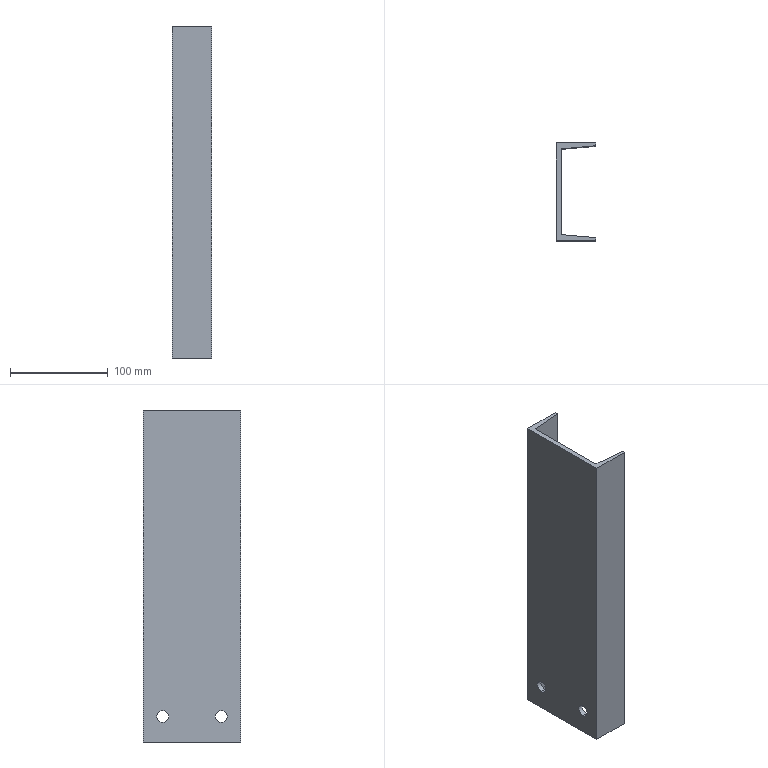Part | STEP file | BCC3 H12_8B | 1 solid | 14 faces | box 40 x 100 x 340 mm | volume 276708 mm3 | plane 10 | cylinder 4 | commonest cylinder face diameters 12 x4
STEP:
#1=CARTESIAN_POINT('',(0.,0.,0.));
#2=DIRECTION('',(0.,0.,1.));
#3=DIRECTION('',(1.,0.,0.));
#4=AXIS2_PLACEMENT_3D('',#1,#2,#3);
#5=CARTESIAN_POINT('',(5.,-30.,-138.));
#6=VERTEX_POINT('',#5);
#7=CARTESIAN_POINT('',(0.,-30.,-138.));
#8=VERTEX_POINT('',#7);
#9=CARTESIAN_POINT('',(10.,-30.,-138.));
#10=DIRECTION('',(-1.,0.,0.));
#11=VECTOR('',#10,1.);
#12=LINE('',#9,#11);
#13=CARTESIAN_POINT('',(10.,-30.,-144.));
#14=DIRECTION('',(-1.,0.,0.));
#15=DIRECTION('',(0.,0.,1.));
#16=AXIS2_PLACEMENT_3D('',#13,#14,#15);
#17=CYLINDRICAL_SURFACE('',#16,6.);
#18=CARTESIAN_POINT('',(6.283,0.));
#19=DIRECTION('',(0.,1.));
#20=VECTOR('',#19,1.);
#21=LINE('',#18,#20);
#22=(GEOMETRIC_REPRESENTATION_CONTEXT(2)PARAMETRIC_REPRESENTATION_CONTEXT()REPRESENTATION_CONTEXT('',''));
#23=DEFINITIONAL_REPRESENTATION('',(#21),#22);
#24=PCURVE('',#17,#23);
#25=CARTESIAN_POINT('',(10.,-30.,-144.));
#26=DIRECTION('',(-1.,0.,0.));
#27=DIRECTION('',(0.,0.,1.));
#28=AXIS2_PLACEMENT_3D('',#25,#26,#27);
#29=CYLINDRICAL_SURFACE('',#28,6.);
#30=CARTESIAN_POINT('',(0.,0.));
#31=DIRECTION('',(0.,1.));
#32=VECTOR('',#31,1.);
#33=LINE('',#30,#32);
#34=(GEOMETRIC_REPRESENTATION_CONTEXT(2)PARAMETRIC_REPRESENTATION_CONTEXT()REPRESENTATION_CONTEXT('',''));
#35=DEFINITIONAL_REPRESENTATION('',(#33),#34);
#36=PCURVE('',#29,#35);
#37=SURFACE_CURVE('',#12,(#24,#36),.PCURVE_S1.);
#38=EDGE_CURVE('',#6,#8,#37,.T.);
#39=ORIENTED_EDGE('',*,*,#38,.T.);
#40=CARTESIAN_POINT('',(0.,-30.,-150.));
#41=VERTEX_POINT('',#40);
#42=CARTESIAN_POINT('',(0.,-30.,-144.));
#43=DIRECTION('',(-1.,0.,0.));
#44=DIRECTION('',(0.,0.,1.));
#45=AXIS2_PLACEMENT_3D('',#42,#43,#44);
#46=CIRCLE('',#45,6.);
#47=CARTESIAN_POINT('',(0.,10.));
#48=DIRECTION('',(1.,0.));
#49=VECTOR('',#48,1.);
#50=LINE('',#47,#49);
#51=(GEOMETRIC_REPRESENTATION_CONTEXT(2)PARAMETRIC_REPRESENTATION_CONTEXT()REPRESENTATION_CONTEXT('',''));
#52=DEFINITIONAL_REPRESENTATION('',(#50),#51);
#53=PCURVE('',#17,#52);
#54=CARTESIAN_POINT('',(0.,50.,170.));
#55=DIRECTION('',(1.,0.,0.));
#56=DIRECTION('',(0.,0.,-1.));
#57=AXIS2_PLACEMENT_3D('',#54,#55,#56);
#58=PLANE('',#57);
#59=CARTESIAN_POINT('',(308.,-80.));
#60=CARTESIAN_POINT('',(308.,-69.608));
#61=CARTESIAN_POINT('',(317.,-74.804));
#62=CARTESIAN_POINT('',(326.,-80.));
#63=CARTESIAN_POINT('',(317.,-85.196));
#64=CARTESIAN_POINT('',(308.,-90.392));
#65=CARTESIAN_POINT('',(308.,-80.));
#66=(BOUNDED_CURVE()B_SPLINE_CURVE(2,(#59,#60,#61,#62,#63,#64,#65),.UNSPECIFIED.,.T.,.F.)B_SPLINE_CURVE_WITH_KNOTS((1,2,2,2,2,1),(-2.094,0.,2.094,4.189,6.283,8.378),.UNSPECIFIED.)CURVE()GEOMETRIC_REPRESENTATION_ITEM()RATIONAL_B_SPLINE_CURVE((1.,0.5,1.,0.5,1.,0.5,1.))REPRESENTATION_ITEM(''));
#67=(GEOMETRIC_REPRESENTATION_CONTEXT(2)PARAMETRIC_REPRESENTATION_CONTEXT()REPRESENTATION_CONTEXT('',''));
#68=DEFINITIONAL_REPRESENTATION('',(#66),#67);
#69=PCURVE('',#58,#68);
#70=SURFACE_CURVE('',#46,(#53,#69),.PCURVE_S1.);
#71=EDGE_CURVE('',#41,#8,#70,.T.);
#72=ORIENTED_EDGE('',*,*,#71,.F.);
#73=CARTESIAN_POINT('',(5.,-30.,-150.));
#74=VERTEX_POINT('',#73);
#75=CARTESIAN_POINT('',(10.,-30.,-150.));
#76=DIRECTION('',(-1.,0.,0.));
#77=VECTOR('',#76,1.);
#78=LINE('',#75,#77);
#79=CARTESIAN_POINT('',(3.142,0.));
#80=DIRECTION('',(0.,1.));
#81=VECTOR('',#80,1.);
#82=LINE('',#79,#81);
#83=(GEOMETRIC_REPRESENTATION_CONTEXT(2)PARAMETRIC_REPRESENTATION_CONTEXT()REPRESENTATION_CONTEXT('',''));
#84=DEFINITIONAL_REPRESENTATION('',(#82),#83);
#85=PCURVE('',#17,#84);
#86=CARTESIAN_POINT('',(3.142,0.));
#87=DIRECTION('',(0.,1.));
#88=VECTOR('',#87,1.);
#89=LINE('',#86,#88);
#90=(GEOMETRIC_REPRESENTATION_CONTEXT(2)PARAMETRIC_REPRESENTATION_CONTEXT()REPRESENTATION_CONTEXT('',''));
#91=DEFINITIONAL_REPRESENTATION('',(#89),#90);
#92=PCURVE('',#29,#91);
#93=SURFACE_CURVE('',#78,(#85,#92),.PCURVE_S1.);
#94=EDGE_CURVE('',#74,#41,#93,.T.);
#95=ORIENTED_EDGE('',*,*,#94,.F.);
#96=CARTESIAN_POINT('',(5.,-30.,-144.));
#97=DIRECTION('',(-1.,0.,0.));
#98=DIRECTION('',(0.,0.,1.));
#99=AXIS2_PLACEMENT_3D('',#96,#97,#98);
#100=CIRCLE('',#99,6.);
#101=CARTESIAN_POINT('',(0.,5.));
#102=DIRECTION('',(1.,0.));
#103=VECTOR('',#102,1.);
#104=LINE('',#101,#103);
#105=(GEOMETRIC_REPRESENTATION_CONTEXT(2)PARAMETRIC_REPRESENTATION_CONTEXT()REPRESENTATION_CONTEXT('',''));
#106=DEFINITIONAL_REPRESENTATION('',(#104),#105);
#107=PCURVE('',#17,#106);
#108=CARTESIAN_POINT('',(5.,-43.938,170.));
#109=DIRECTION('',(-1.,0.,0.));
#110=DIRECTION('',(0.,0.,1.));
#111=AXIS2_PLACEMENT_3D('',#108,#109,#110);
#112=PLANE('',#111);
#113=CARTESIAN_POINT('',(-314.,13.938));
#114=DIRECTION('',(1.,0.));
#115=AXIS2_PLACEMENT_2D('',#113,#114);
#116=CIRCLE('',#115,6.);
#117=(GEOMETRIC_REPRESENTATION_CONTEXT(2)PARAMETRIC_REPRESENTATION_CONTEXT()REPRESENTATION_CONTEXT('',''));
#118=DEFINITIONAL_REPRESENTATION('',(#116),#117);
#119=PCURVE('',#112,#118);
#120=SURFACE_CURVE('',#100,(#107,#119),.PCURVE_S1.);
#121=EDGE_CURVE('',#74,#6,#120,.T.);
#122=ORIENTED_EDGE('',*,*,#121,.T.);
#123=EDGE_LOOP('',(#39,#72,#95,#122));
#124=FACE_BOUND('',#123,.F.);
#125=ADVANCED_FACE('',(#124),#17,.F.);
#126=CARTESIAN_POINT('',(5.,30.,-138.));
#127=VERTEX_POINT('',#126);
#128=CARTESIAN_POINT('',(0.,30.,-138.));
#129=VERTEX_POINT('',#128);
#130=CARTESIAN_POINT('',(10.,30.,-138.));
#131=DIRECTION('',(-1.,0.,0.));
#132=VECTOR('',#131,1.);
#133=LINE('',#130,#132);
#134=CARTESIAN_POINT('',(10.,30.,-144.));
#135=DIRECTION('',(-1.,0.,0.));
#136=DIRECTION('',(0.,0.,1.));
#137=AXIS2_PLACEMENT_3D('',#134,#135,#136);
#138=CYLINDRICAL_SURFACE('',#137,6.);
#139=CARTESIAN_POINT('',(6.283,0.));
#140=DIRECTION('',(0.,1.));
#141=VECTOR('',#140,1.);
#142=LINE('',#139,#141);
#143=(GEOMETRIC_REPRESENTATION_CONTEXT(2)PARAMETRIC_REPRESENTATION_CONTEXT()REPRESENTATION_CONTEXT('',''));
#144=DEFINITIONAL_REPRESENTATION('',(#142),#143);
#145=PCURVE('',#138,#144);
#146=CARTESIAN_POINT('',(10.,30.,-144.));
#147=DIRECTION('',(-1.,0.,0.));
#148=DIRECTION('',(0.,0.,1.));
#149=AXIS2_PLACEMENT_3D('',#146,#147,#148);
#150=CYLINDRICAL_SURFACE('',#149,6.);
#151=CARTESIAN_POINT('',(0.,0.));
#152=DIRECTION('',(0.,1.));
#153=VECTOR('',#152,1.);
#154=LINE('',#151,#153);
#155=(GEOMETRIC_REPRESENTATION_CONTEXT(2)PARAMETRIC_REPRESENTATION_CONTEXT()REPRESENTATION_CONTEXT('',''));
#156=DEFINITIONAL_REPRESENTATION('',(#154),#155);
#157=PCURVE('',#150,#156);
#158=SURFACE_CURVE('',#133,(#145,#157),.PCURVE_S1.);
#159=EDGE_CURVE('',#127,#129,#158,.T.);
#160=ORIENTED_EDGE('',*,*,#159,.T.);
#161=CARTESIAN_POINT('',(0.,30.,-150.));
#162=VERTEX_POINT('',#161);
#163=CARTESIAN_POINT('',(0.,30.,-144.));
#164=DIRECTION('',(-1.,0.,0.));
#165=DIRECTION('',(0.,0.,1.));
#166=AXIS2_PLACEMENT_3D('',#163,#164,#165);
#167=CIRCLE('',#166,6.);
#168=CARTESIAN_POINT('',(0.,10.));
#169=DIRECTION('',(1.,0.));
#170=VECTOR('',#169,1.);
#171=LINE('',#168,#170);
#172=(GEOMETRIC_REPRESENTATION_CONTEXT(2)PARAMETRIC_REPRESENTATION_CONTEXT()REPRESENTATION_CONTEXT('',''));
#173=DEFINITIONAL_REPRESENTATION('',(#171),#172);
#174=PCURVE('',#138,#173);
#175=CARTESIAN_POINT('',(308.,-20.));
#176=CARTESIAN_POINT('',(308.,-9.608));
#177=CARTESIAN_POINT('',(317.,-14.804));
#178=CARTESIAN_POINT('',(326.,-20.));
#179=CARTESIAN_POINT('',(317.,-25.196));
#180=CARTESIAN_POINT('',(308.,-30.392));
#181=CARTESIAN_POINT('',(308.,-20.));
#182=(BOUNDED_CURVE()B_SPLINE_CURVE(2,(#175,#176,#177,#178,#179,#180,#181),.UNSPECIFIED.,.T.,.F.)B_SPLINE_CURVE_WITH_KNOTS((1,2,2,2,2,1),(-2.094,0.,2.094,4.189,6.283,8.378),.UNSPECIFIED.)CURVE()GEOMETRIC_REPRESENTATION_ITEM()RATIONAL_B_SPLINE_CURVE((1.,0.5,1.,0.5,1.,0.5,1.))REPRESENTATION_ITEM(''));
#183=(GEOMETRIC_REPRESENTATION_CONTEXT(2)PARAMETRIC_REPRESENTATION_CONTEXT()REPRESENTATION_CONTEXT('',''));
#184=DEFINITIONAL_REPRESENTATION('',(#182),#183);
#185=PCURVE('',#58,#184);
#186=SURFACE_CURVE('',#167,(#174,#185),.PCURVE_S1.);
#187=EDGE_CURVE('',#162,#129,#186,.T.);
#188=ORIENTED_EDGE('',*,*,#187,.F.);
#189=CARTESIAN_POINT('',(5.,30.,-150.));
#190=VERTEX_POINT('',#189);
#191=CARTESIAN_POINT('',(10.,30.,-150.));
#192=DIRECTION('',(-1.,0.,0.));
#193=VECTOR('',#192,1.);
#194=LINE('',#191,#193);
#195=CARTESIAN_POINT('',(3.142,0.));
#196=DIRECTION('',(0.,1.));
#197=VECTOR('',#196,1.);
#198=LINE('',#195,#197);
#199=(GEOMETRIC_REPRESENTATION_CONTEXT(2)PARAMETRIC_REPRESENTATION_CONTEXT()REPRESENTATION_CONTEXT('',''));
#200=DEFINITIONAL_REPRESENTATION('',(#198),#199);
#201=PCURVE('',#138,#200);
#202=CARTESIAN_POINT('',(3.142,0.));
#203=DIRECTION('',(0.,1.));
#204=VECTOR('',#203,1.);
#205=LINE('',#202,#204);
#206=(GEOMETRIC_REPRESENTATION_CONTEXT(2)PARAMETRIC_REPRESENTATION_CONTEXT()REPRESENTATION_CONTEXT('',''));
#207=DEFINITIONAL_REPRESENTATION('',(#205),#206);
#208=PCURVE('',#150,#207);
#209=SURFACE_CURVE('',#194,(#201,#208),.PCURVE_S1.);
#210=EDGE_CURVE('',#190,#162,#209,.T.);
#211=ORIENTED_EDGE('',*,*,#210,.F.);
#212=CARTESIAN_POINT('',(5.,30.,-144.));
#213=DIRECTION('',(-1.,0.,0.));
#214=DIRECTION('',(0.,0.,1.));
#215=AXIS2_PLACEMENT_3D('',#212,#213,#214);
#216=CIRCLE('',#215,6.);
#217=CARTESIAN_POINT('',(0.,5.));
#218=DIRECTION('',(1.,0.));
#219=VECTOR('',#218,1.);
#220=LINE('',#217,#219);
#221=(GEOMETRIC_REPRESENTATION_CONTEXT(2)PARAMETRIC_REPRESENTATION_CONTEXT()REPRESENTATION_CONTEXT('',''));
#222=DEFINITIONAL_REPRESENTATION('',(#220),#221);
#223=PCURVE('',#138,#222);
#224=CARTESIAN_POINT('',(-314.,73.938));
#225=DIRECTION('',(1.,0.));
#226=AXIS2_PLACEMENT_2D('',#224,#225);
#227=CIRCLE('',#226,6.);
#228=(GEOMETRIC_REPRESENTATION_CONTEXT(2)PARAMETRIC_REPRESENTATION_CONTEXT()REPRESENTATION_CONTEXT('',''));
#229=DEFINITIONAL_REPRESENTATION('',(#227),#228);
#230=PCURVE('',#112,#229);
#231=SURFACE_CURVE('',#216,(#223,#230),.PCURVE_S1.);
#232=EDGE_CURVE('',#190,#127,#231,.T.);
#233=ORIENTED_EDGE('',*,*,#232,.T.);
#234=EDGE_LOOP('',(#160,#188,#211,#233));
#235=FACE_BOUND('',#234,.F.);
#236=ADVANCED_FACE('',(#235),#138,.F.);
#237=CARTESIAN_POINT('',(40.,50.,-170.));
#238=VERTEX_POINT('',#237);
#239=CARTESIAN_POINT('',(0.,50.,-170.));
#240=VERTEX_POINT('',#239);
#241=CARTESIAN_POINT('',(40.,50.,-170.));
#242=DIRECTION('',(-1.,0.,0.));
#243=VECTOR('',#242,1.);
#244=LINE('',#241,#243);
#245=CARTESIAN_POINT('',(40.,50.,170.));
#246=DIRECTION('',(0.,-1.,0.));
#247=DIRECTION('',(1.,0.,0.));
#248=AXIS2_PLACEMENT_3D('',#245,#246,#247);
#249=PLANE('',#248);
#250=CARTESIAN_POINT('',(0.,-340.));
#251=DIRECTION('',(-1.,0.));
#252=VECTOR('',#251,1.);
#253=LINE('',#250,#252);
#254=(GEOMETRIC_REPRESENTATION_CONTEXT(2)PARAMETRIC_REPRESENTATION_CONTEXT()REPRESENTATION_CONTEXT('',''));
#255=DEFINITIONAL_REPRESENTATION('',(#253),#254);
#256=PCURVE('',#249,#255);
#257=CARTESIAN_POINT('',(0.,0.,-170.));
#258=DIRECTION('',(0.,0.,1.));
#259=DIRECTION('',(1.,0.,0.));
#260=AXIS2_PLACEMENT_3D('',#257,#258,#259);
#261=PLANE('',#260);
#262=CARTESIAN_POINT('',(40.,50.));
#263=DIRECTION('',(-1.,0.));
#264=VECTOR('',#263,1.);
#265=LINE('',#262,#264);
#266=(GEOMETRIC_REPRESENTATION_CONTEXT(2)PARAMETRIC_REPRESENTATION_CONTEXT()REPRESENTATION_CONTEXT('',''));
#267=DEFINITIONAL_REPRESENTATION('',(#265),#266);
#268=PCURVE('',#261,#267);
#269=SURFACE_CURVE('',#244,(#256,#268),.PCURVE_S1.);
#270=EDGE_CURVE('',#238,#240,#269,.T.);
#271=ORIENTED_EDGE('',*,*,#270,.T.);
#272=CARTESIAN_POINT('',(0.,50.,170.));
#273=VERTEX_POINT('',#272);
#274=CARTESIAN_POINT('',(0.,50.,170.));
#275=DIRECTION('',(0.,0.,-1.));
#276=VECTOR('',#275,1.);
#277=LINE('',#274,#276);
#278=CARTESIAN_POINT('',(-40.,0.));
#279=DIRECTION('',(0.,-1.));
#280=VECTOR('',#279,1.);
#281=LINE('',#278,#280);
#282=(GEOMETRIC_REPRESENTATION_CONTEXT(2)PARAMETRIC_REPRESENTATION_CONTEXT()REPRESENTATION_CONTEXT('',''));
#283=DEFINITIONAL_REPRESENTATION('',(#281),#282);
#284=PCURVE('',#249,#283);
#285=CARTESIAN_POINT('',(0.,0.));
#286=DIRECTION('',(1.,0.));
#287=VECTOR('',#286,1.);
#288=LINE('',#285,#287);
#289=(GEOMETRIC_REPRESENTATION_CONTEXT(2)PARAMETRIC_REPRESENTATION_CONTEXT()REPRESENTATION_CONTEXT('',''));
#290=DEFINITIONAL_REPRESENTATION('',(#288),#289);
#291=PCURVE('',#58,#290);
#292=SURFACE_CURVE('',#277,(#284,#291),.PCURVE_S1.);
#293=EDGE_CURVE('',#273,#240,#292,.T.);
#294=ORIENTED_EDGE('',*,*,#293,.F.);
#295=CARTESIAN_POINT('',(40.,50.,170.));
#296=VERTEX_POINT('',#295);
#297=CARTESIAN_POINT('',(40.,50.,170.));
#298=DIRECTION('',(-1.,0.,0.));
#299=VECTOR('',#298,1.);
#300=LINE('',#297,#299);
#301=CARTESIAN_POINT('',(0.,0.));
#302=DIRECTION('',(-1.,0.));
#303=VECTOR('',#302,1.);
#304=LINE('',#301,#303);
#305=(GEOMETRIC_REPRESENTATION_CONTEXT(2)PARAMETRIC_REPRESENTATION_CONTEXT()REPRESENTATION_CONTEXT('',''));
#306=DEFINITIONAL_REPRESENTATION('',(#304),#305);
#307=PCURVE('',#249,#306);
#308=CARTESIAN_POINT('',(0.,0.,170.));
#309=DIRECTION('',(0.,0.,1.));
#310=DIRECTION('',(1.,0.,0.));
#311=AXIS2_PLACEMENT_3D('',#308,#309,#310);
#312=PLANE('',#311);
#313=CARTESIAN_POINT('',(40.,50.));
#314=DIRECTION('',(-1.,0.));
#315=VECTOR('',#314,1.);
#316=LINE('',#313,#315);
#317=(GEOMETRIC_REPRESENTATION_CONTEXT(2)PARAMETRIC_REPRESENTATION_CONTEXT()REPRESENTATION_CONTEXT('',''));
#318=DEFINITIONAL_REPRESENTATION('',(#316),#317);
#319=PCURVE('',#312,#318);
#320=SURFACE_CURVE('',#300,(#307,#319),.PCURVE_S1.);
#321=EDGE_CURVE('',#296,#273,#320,.T.);
#322=ORIENTED_EDGE('',*,*,#321,.F.);
#323=CARTESIAN_POINT('',(40.,50.,170.));
#324=DIRECTION('',(0.,0.,-1.));
#325=VECTOR('',#324,1.);
#326=LINE('',#323,#325);
#327=CARTESIAN_POINT('',(0.,0.));
#328=DIRECTION('',(0.,-1.));
#329=VECTOR('',#328,1.);
#330=LINE('',#327,#329);
#331=(GEOMETRIC_REPRESENTATION_CONTEXT(2)PARAMETRIC_REPRESENTATION_CONTEXT()REPRESENTATION_CONTEXT('',''));
#332=DEFINITIONAL_REPRESENTATION('',(#330),#331);
#333=PCURVE('',#249,#332);
#334=CARTESIAN_POINT('',(40.,47.,170.));
#335=DIRECTION('',(-1.,0.,0.));
#336=DIRECTION('',(0.,-1.,0.));
#337=AXIS2_PLACEMENT_3D('',#334,#335,#336);
#338=PLANE('',#337);
#339=CARTESIAN_POINT('',(-3.,0.));
#340=DIRECTION('',(0.,-1.));
#341=VECTOR('',#340,1.);
#342=LINE('',#339,#341);
#343=(GEOMETRIC_REPRESENTATION_CONTEXT(2)PARAMETRIC_REPRESENTATION_CONTEXT()REPRESENTATION_CONTEXT('',''));
#344=DEFINITIONAL_REPRESENTATION('',(#342),#343);
#345=PCURVE('',#338,#344);
#346=SURFACE_CURVE('',#326,(#333,#345),.PCURVE_S1.);
#347=EDGE_CURVE('',#296,#238,#346,.T.);
#348=ORIENTED_EDGE('',*,*,#347,.T.);
#349=EDGE_LOOP('',(#271,#294,#322,#348));
#350=FACE_BOUND('',#349,.T.);
#351=ADVANCED_FACE('',(#350),#249,.F.);
#352=CARTESIAN_POINT('',(0.,-30.,-144.));
#353=DIRECTION('',(-1.,0.,0.));
#354=DIRECTION('',(0.,0.,1.));
#355=AXIS2_PLACEMENT_3D('',#352,#353,#354);
#356=CIRCLE('',#355,6.);
#357=CARTESIAN_POINT('',(308.,-80.));
#358=CARTESIAN_POINT('',(308.,-69.608));
#359=CARTESIAN_POINT('',(317.,-74.804));
#360=CARTESIAN_POINT('',(326.,-80.));
#361=CARTESIAN_POINT('',(317.,-85.196));
#362=CARTESIAN_POINT('',(308.,-90.392));
#363=CARTESIAN_POINT('',(308.,-80.));
#364=(BOUNDED_CURVE()B_SPLINE_CURVE(2,(#357,#358,#359,#360,#361,#362,#363),.UNSPECIFIED.,.T.,.F.)B_SPLINE_CURVE_WITH_KNOTS((1,2,2,2,2,1),(-2.094,0.,2.094,4.189,6.283,8.378),.UNSPECIFIED.)CURVE()GEOMETRIC_REPRESENTATION_ITEM()RATIONAL_B_SPLINE_CURVE((1.,0.5,1.,0.5,1.,0.5,1.))REPRESENTATION_ITEM(''));
#365=(GEOMETRIC_REPRESENTATION_CONTEXT(2)PARAMETRIC_REPRESENTATION_CONTEXT()REPRESENTATION_CONTEXT('',''));
#366=DEFINITIONAL_REPRESENTATION('',(#364),#365);
#367=PCURVE('',#58,#366);
#368=CARTESIAN_POINT('',(0.,10.));
#369=DIRECTION('',(1.,0.));
#370=VECTOR('',#369,1.);
#371=LINE('',#368,#370);
#372=(GEOMETRIC_REPRESENTATION_CONTEXT(2)PARAMETRIC_REPRESENTATION_CONTEXT()REPRESENTATION_CONTEXT('',''));
#373=DEFINITIONAL_REPRESENTATION('',(#371),#372);
#374=PCURVE('',#29,#373);
#375=SURFACE_CURVE('',#356,(#367,#374),.PCURVE_S1.);
#376=EDGE_CURVE('',#8,#41,#375,.T.);
#377=ORIENTED_EDGE('',*,*,#376,.F.);
#378=ORIENTED_EDGE('',*,*,#71,.F.);
#379=EDGE_LOOP('',(#377,#378));
#380=FACE_BOUND('',#379,.T.);
#381=CARTESIAN_POINT('',(0.,30.,-144.));
#382=DIRECTION('',(-1.,0.,0.));
#383=DIRECTION('',(0.,0.,1.));
#384=AXIS2_PLACEMENT_3D('',#381,#382,#383);
#385=CIRCLE('',#384,6.);
#386=CARTESIAN_POINT('',(308.,-20.));
#387=CARTESIAN_POINT('',(308.,-9.608));
#388=CARTESIAN_POINT('',(317.,-14.804));
#389=CARTESIAN_POINT('',(326.,-20.));
#390=CARTESIAN_POINT('',(317.,-25.196));
#391=CARTESIAN_POINT('',(308.,-30.392));
#392=CARTESIAN_POINT('',(308.,-20.));
#393=(BOUNDED_CURVE()B_SPLINE_CURVE(2,(#386,#387,#388,#389,#390,#391,#392),.UNSPECIFIED.,.T.,.F.)B_SPLINE_CURVE_WITH_KNOTS((1,2,2,2,2,1),(-2.094,0.,2.094,4.189,6.283,8.378),.UNSPECIFIED.)CURVE()GEOMETRIC_REPRESENTATION_ITEM()RATIONAL_B_SPLINE_CURVE((1.,0.5,1.,0.5,1.,0.5,1.))REPRESENTATION_ITEM(''));
#394=(GEOMETRIC_REPRESENTATION_CONTEXT(2)PARAMETRIC_REPRESENTATION_CONTEXT()REPRESENTATION_CONTEXT('',''));
#395=DEFINITIONAL_REPRESENTATION('',(#393),#394);
#396=PCURVE('',#58,#395);
#397=CARTESIAN_POINT('',(0.,10.));
#398=DIRECTION('',(1.,0.));
#399=VECTOR('',#398,1.);
#400=LINE('',#397,#399);
#401=(GEOMETRIC_REPRESENTATION_CONTEXT(2)PARAMETRIC_REPRESENTATION_CONTEXT()REPRESENTATION_CONTEXT('',''));
#402=DEFINITIONAL_REPRESENTATION('',(#400),#401);
#403=PCURVE('',#150,#402);
#404=SURFACE_CURVE('',#385,(#396,#403),.PCURVE_S1.);
#405=EDGE_CURVE('',#129,#162,#404,.T.);
#406=ORIENTED_EDGE('',*,*,#405,.F.);
#407=ORIENTED_EDGE('',*,*,#187,.F.);
#408=EDGE_LOOP('',(#406,#407));
#409=FACE_BOUND('',#408,.T.);
#410=CARTESIAN_POINT('',(0.,-50.,-170.));
#411=VERTEX_POINT('',#410);
#412=CARTESIAN_POINT('',(0.,50.,-170.));
#413=DIRECTION('',(0.,-1.,0.));
#414=VECTOR('',#413,1.);
#415=LINE('',#412,#414);
#416=CARTESIAN_POINT('',(340.,0.));
#417=DIRECTION('',(0.,-1.));
#418=VECTOR('',#417,1.);
#419=LINE('',#416,#418);
#420=(GEOMETRIC_REPRESENTATION_CONTEXT(2)PARAMETRIC_REPRESENTATION_CONTEXT()REPRESENTATION_CONTEXT('',''));
#421=DEFINITIONAL_REPRESENTATION('',(#419),#420);
#422=PCURVE('',#58,#421);
#423=CARTESIAN_POINT('',(0.,50.));
#424=DIRECTION('',(0.,-1.));
#425=VECTOR('',#424,1.);
#426=LINE('',#423,#425);
#427=(GEOMETRIC_REPRESENTATION_CONTEXT(2)PARAMETRIC_REPRESENTATION_CONTEXT()REPRESENTATION_CONTEXT('',''));
#428=DEFINITIONAL_REPRESENTATION('',(#426),#427);
#429=PCURVE('',#261,#428);
#430=SURFACE_CURVE('',#415,(#422,#429),.PCURVE_S1.);
#431=EDGE_CURVE('',#240,#411,#430,.T.);
#432=ORIENTED_EDGE('',*,*,#431,.T.);
#433=CARTESIAN_POINT('',(0.,-50.,170.));
#434=VERTEX_POINT('',#433);
#435=CARTESIAN_POINT('',(0.,-50.,170.));
#436=DIRECTION('',(0.,0.,-1.));
#437=VECTOR('',#436,1.);
#438=LINE('',#435,#437);
#439=CARTESIAN_POINT('',(0.,-100.));
#440=DIRECTION('',(1.,0.));
#441=VECTOR('',#440,1.);
#442=LINE('',#439,#441);
#443=(GEOMETRIC_REPRESENTATION_CONTEXT(2)PARAMETRIC_REPRESENTATION_CONTEXT()REPRESENTATION_CONTEXT('',''));
#444=DEFINITIONAL_REPRESENTATION('',(#442),#443);
#445=PCURVE('',#58,#444);
#446=CARTESIAN_POINT('',(0.,-50.,170.));
#447=DIRECTION('',(0.,1.,0.));
#448=DIRECTION('',(-1.,0.,0.));
#449=AXIS2_PLACEMENT_3D('',#446,#447,#448);
#450=PLANE('',#449);
#451=CARTESIAN_POINT('',(0.,0.));
#452=DIRECTION('',(0.,-1.));
#453=VECTOR('',#452,1.);
#454=LINE('',#451,#453);
#455=(GEOMETRIC_REPRESENTATION_CONTEXT(2)PARAMETRIC_REPRESENTATION_CONTEXT()REPRESENTATION_CONTEXT('',''));
#456=DEFINITIONAL_REPRESENTATION('',(#454),#455);
#457=PCURVE('',#450,#456);
#458=SURFACE_CURVE('',#438,(#445,#457),.PCURVE_S1.);
#459=EDGE_CURVE('',#434,#411,#458,.T.);
#460=ORIENTED_EDGE('',*,*,#459,.F.);
#461=CARTESIAN_POINT('',(0.,50.,170.));
#462=DIRECTION('',(0.,-1.,0.));
#463=VECTOR('',#462,1.);
#464=LINE('',#461,#463);
#465=CARTESIAN_POINT('',(0.,0.));
#466=DIRECTION('',(0.,-1.));
#467=VECTOR('',#466,1.);
#468=LINE('',#465,#467);
#469=(GEOMETRIC_REPRESENTATION_CONTEXT(2)PARAMETRIC_REPRESENTATION_CONTEXT()REPRESENTATION_CONTEXT('',''));
#470=DEFINITIONAL_REPRESENTATION('',(#468),#469);
#471=PCURVE('',#58,#470);
#472=CARTESIAN_POINT('',(0.,50.));
#473=DIRECTION('',(0.,-1.));
#474=VECTOR('',#473,1.);
#475=LINE('',#472,#474);
#476=(GEOMETRIC_REPRESENTATION_CONTEXT(2)PARAMETRIC_REPRESENTATION_CONTEXT()REPRESENTATION_CONTEXT('',''));
#477=DEFINITIONAL_REPRESENTATION('',(#475),#476);
#478=PCURVE('',#312,#477);
#479=SURFACE_CURVE('',#464,(#471,#478),.PCURVE_S1.);
#480=EDGE_CURVE('',#273,#434,#479,.T.);
#481=ORIENTED_EDGE('',*,*,#480,.F.);
#482=ORIENTED_EDGE('',*,*,#293,.T.);
#483=EDGE_LOOP('',(#432,#460,#481,#482));
#484=FACE_BOUND('',#483,.T.);
#485=ADVANCED_FACE('',(#380,#409,#484),#58,.F.);
#486=CARTESIAN_POINT('',(40.,-50.,-170.));
#487=VERTEX_POINT('',#486);
#488=CARTESIAN_POINT('',(0.,-50.,-170.));
#489=DIRECTION('',(1.,0.,0.));
#490=VECTOR('',#489,1.);
#491=LINE('',#488,#490);
#492=CARTESIAN_POINT('',(0.,-340.));
#493=DIRECTION('',(-1.,0.));
#494=VECTOR('',#493,1.);
#495=LINE('',#492,#494);
#496=(GEOMETRIC_REPRESENTATION_CONTEXT(2)PARAMETRIC_REPRESENTATION_CONTEXT()REPRESENTATION_CONTEXT('',''));
#497=DEFINITIONAL_REPRESENTATION('',(#495),#496);
#498=PCURVE('',#450,#497);
#499=CARTESIAN_POINT('',(0.,-50.));
#500=DIRECTION('',(1.,0.));
#501=VECTOR('',#500,1.);
#502=LINE('',#499,#501);
#503=(GEOMETRIC_REPRESENTATION_CONTEXT(2)PARAMETRIC_REPRESENTATION_CONTEXT()REPRESENTATION_CONTEXT('',''));
#504=DEFINITIONAL_REPRESENTATION('',(#502),#503);
#505=PCURVE('',#261,#504);
#506=SURFACE_CURVE('',#491,(#498,#505),.PCURVE_S1.);
#507=EDGE_CURVE('',#411,#487,#506,.T.);
#508=ORIENTED_EDGE('',*,*,#507,.T.);
#509=CARTESIAN_POINT('',(40.,-50.,170.));
#510=VERTEX_POINT('',#509);
#511=CARTESIAN_POINT('',(40.,-50.,170.));
#512=DIRECTION('',(0.,0.,-1.));
#513=VECTOR('',#512,1.);
#514=LINE('',#511,#513);
#515=CARTESIAN_POINT('',(-40.,0.));
#516=DIRECTION('',(0.,-1.));
#517=VECTOR('',#516,1.);
#518=LINE('',#515,#517);
#519=(GEOMETRIC_REPRESENTATION_CONTEXT(2)PARAMETRIC_REPRESENTATION_CONTEXT()REPRESENTATION_CONTEXT('',''));
#520=DEFINITIONAL_REPRESENTATION('',(#518),#519);
#521=PCURVE('',#450,#520);
#522=CARTESIAN_POINT('',(40.,-50.,170.));
#523=DIRECTION('',(-1.,0.,0.));
#524=DIRECTION('',(0.,-1.,0.));
#525=AXIS2_PLACEMENT_3D('',#522,#523,#524);
#526=PLANE('',#525);
#527=CARTESIAN_POINT('',(0.,0.));
#528=DIRECTION('',(0.,-1.));
#529=VECTOR('',#528,1.);
#530=LINE('',#527,#529);
#531=(GEOMETRIC_REPRESENTATION_CONTEXT(2)PARAMETRIC_REPRESENTATION_CONTEXT()REPRESENTATION_CONTEXT('',''));
#532=DEFINITIONAL_REPRESENTATION('',(#530),#531);
#533=PCURVE('',#526,#532);
#534=SURFACE_CURVE('',#514,(#521,#533),.PCURVE_S1.);
#535=EDGE_CURVE('',#510,#487,#534,.T.);
#536=ORIENTED_EDGE('',*,*,#535,.F.);
#537=CARTESIAN_POINT('',(0.,-50.,170.));
#538=DIRECTION('',(1.,0.,0.));
#539=VECTOR('',#538,1.);
#540=LINE('',#537,#539);
#541=CARTESIAN_POINT('',(0.,0.));
#542=DIRECTION('',(-1.,0.));
#543=VECTOR('',#542,1.);
#544=LINE('',#541,#543);
#545=(GEOMETRIC_REPRESENTATION_CONTEXT(2)PARAMETRIC_REPRESENTATION_CONTEXT()REPRESENTATION_CONTEXT('',''));
#546=DEFINITIONAL_REPRESENTATION('',(#544),#545);
#547=PCURVE('',#450,#546);
#548=CARTESIAN_POINT('',(0.,-50.));
#549=DIRECTION('',(1.,0.));
#550=VECTOR('',#549,1.);
#551=LINE('',#548,#550);
#552=(GEOMETRIC_REPRESENTATION_CONTEXT(2)PARAMETRIC_REPRESENTATION_CONTEXT()REPRESENTATION_CONTEXT('',''));
#553=DEFINITIONAL_REPRESENTATION('',(#551),#552);
#554=PCURVE('',#312,#553);
#555=SURFACE_CURVE('',#540,(#547,#554),.PCURVE_S1.);
#556=EDGE_CURVE('',#434,#510,#555,.T.);
#557=ORIENTED_EDGE('',*,*,#556,.F.);
#558=ORIENTED_EDGE('',*,*,#459,.T.);
#559=EDGE_LOOP('',(#508,#536,#557,#558));
#560=FACE_BOUND('',#559,.T.);
#561=ADVANCED_FACE('',(#560),#450,.F.);
#562=CARTESIAN_POINT('',(40.,-47.,-170.));
#563=VERTEX_POINT('',#562);
#564=CARTESIAN_POINT('',(40.,-50.,-170.));
#565=DIRECTION('',(0.,1.,0.));
#566=VECTOR('',#565,1.);
#567=LINE('',#564,#566);
#568=CARTESIAN_POINT('',(0.,-340.));
#569=DIRECTION('',(-1.,0.));
#570=VECTOR('',#569,1.);
#571=LINE('',#568,#570);
#572=(GEOMETRIC_REPRESENTATION_CONTEXT(2)PARAMETRIC_REPRESENTATION_CONTEXT()REPRESENTATION_CONTEXT('',''));
#573=DEFINITIONAL_REPRESENTATION('',(#571),#572);
#574=PCURVE('',#526,#573);
#575=CARTESIAN_POINT('',(40.,-50.));
#576=DIRECTION('',(0.,1.));
#577=VECTOR('',#576,1.);
#578=LINE('',#575,#577);
#579=(GEOMETRIC_REPRESENTATION_CONTEXT(2)PARAMETRIC_REPRESENTATION_CONTEXT()REPRESENTATION_CONTEXT('',''));
#580=DEFINITIONAL_REPRESENTATION('',(#578),#579);
#581=PCURVE('',#261,#580);
#582=SURFACE_CURVE('',#567,(#574,#581),.PCURVE_S1.);
#583=EDGE_CURVE('',#487,#563,#582,.T.);
#584=ORIENTED_EDGE('',*,*,#583,.T.);
#585=CARTESIAN_POINT('',(40.,-47.,170.));
#586=VERTEX_POINT('',#585);
#587=CARTESIAN_POINT('',(40.,-47.,170.));
#588=DIRECTION('',(0.,0.,-1.));
#589=VECTOR('',#588,1.);
#590=LINE('',#587,#589);
#591=CARTESIAN_POINT('',(-3.,0.));
#592=DIRECTION('',(0.,-1.));
#593=VECTOR('',#592,1.);
#594=LINE('',#591,#593);
#595=(GEOMETRIC_REPRESENTATION_CONTEXT(2)PARAMETRIC_REPRESENTATION_CONTEXT()REPRESENTATION_CONTEXT('',''));
#596=DEFINITIONAL_REPRESENTATION('',(#594),#595);
#597=PCURVE('',#526,#596);
#598=CARTESIAN_POINT('',(40.,-47.,170.));
#599=DIRECTION('',(-0.08716,-0.9962,0.));
#600=DIRECTION('',(0.9962,-0.08716,0.));
#601=AXIS2_PLACEMENT_3D('',#598,#599,#600);
#602=PLANE('',#601);
#603=CARTESIAN_POINT('',(0.,0.));
#604=DIRECTION('',(0.,-1.));
#605=VECTOR('',#604,1.);
#606=LINE('',#603,#605);
#607=(GEOMETRIC_REPRESENTATION_CONTEXT(2)PARAMETRIC_REPRESENTATION_CONTEXT()REPRESENTATION_CONTEXT('',''));
#608=DEFINITIONAL_REPRESENTATION('',(#606),#607);
#609=PCURVE('',#602,#608);
#610=SURFACE_CURVE('',#590,(#597,#609),.PCURVE_S1.);
#611=EDGE_CURVE('',#586,#563,#610,.T.);
#612=ORIENTED_EDGE('',*,*,#611,.F.);
#613=CARTESIAN_POINT('',(40.,-50.,170.));
#614=DIRECTION('',(0.,1.,0.));
#615=VECTOR('',#614,1.);
#616=LINE('',#613,#615);
#617=CARTESIAN_POINT('',(0.,0.));
#618=DIRECTION('',(-1.,0.));
#619=VECTOR('',#618,1.);
#620=LINE('',#617,#619);
#621=(GEOMETRIC_REPRESENTATION_CONTEXT(2)PARAMETRIC_REPRESENTATION_CONTEXT()REPRESENTATION_CONTEXT('',''));
#622=DEFINITIONAL_REPRESENTATION('',(#620),#621);
#623=PCURVE('',#526,#622);
#624=CARTESIAN_POINT('',(40.,-50.));
#625=DIRECTION('',(0.,1.));
#626=VECTOR('',#625,1.);
#627=LINE('',#624,#626);
#628=(GEOMETRIC_REPRESENTATION_CONTEXT(2)PARAMETRIC_REPRESENTATION_CONTEXT()REPRESENTATION_CONTEXT('',''));
#629=DEFINITIONAL_REPRESENTATION('',(#627),#628);
#630=PCURVE('',#312,#629);
#631=SURFACE_CURVE('',#616,(#623,#630),.PCURVE_S1.);
#632=EDGE_CURVE('',#510,#586,#631,.T.);
#633=ORIENTED_EDGE('',*,*,#632,.F.);
#634=ORIENTED_EDGE('',*,*,#535,.T.);
#635=EDGE_LOOP('',(#584,#612,#633,#634));
#636=FACE_BOUND('',#635,.T.);
#637=ADVANCED_FACE('',(#636),#526,.F.);
#638=CARTESIAN_POINT('',(5.,-43.938,-170.));
#639=VERTEX_POINT('',#638);
#640=CARTESIAN_POINT('',(40.,-47.,-170.));
#641=DIRECTION('',(-0.9962,0.08716,0.));
#642=VECTOR('',#641,1.);
#643=LINE('',#640,#642);
#644=CARTESIAN_POINT('',(0.,-340.));
#645=DIRECTION('',(-1.,0.));
#646=VECTOR('',#645,1.);
#647=LINE('',#644,#646);
#648=(GEOMETRIC_REPRESENTATION_CONTEXT(2)PARAMETRIC_REPRESENTATION_CONTEXT()REPRESENTATION_CONTEXT('',''));
#649=DEFINITIONAL_REPRESENTATION('',(#647),#648);
#650=PCURVE('',#602,#649);
#651=CARTESIAN_POINT('',(40.,-47.));
#652=DIRECTION('',(-0.9962,0.08716));
#653=VECTOR('',#652,1.);
#654=LINE('',#651,#653);
#655=(GEOMETRIC_REPRESENTATION_CONTEXT(2)PARAMETRIC_REPRESENTATION_CONTEXT()REPRESENTATION_CONTEXT('',''));
#656=DEFINITIONAL_REPRESENTATION('',(#654),#655);
#657=PCURVE('',#261,#656);
#658=SURFACE_CURVE('',#643,(#650,#657),.PCURVE_S1.);
#659=EDGE_CURVE('',#563,#639,#658,.T.);
#660=ORIENTED_EDGE('',*,*,#659,.T.);
#661=CARTESIAN_POINT('',(5.,-43.938,170.));
#662=VERTEX_POINT('',#661);
#663=CARTESIAN_POINT('',(5.,-43.938,170.));
#664=DIRECTION('',(0.,0.,-1.));
#665=VECTOR('',#664,1.);
#666=LINE('',#663,#665);
#667=CARTESIAN_POINT('',(-35.134,0.));
#668=DIRECTION('',(0.,-1.));
#669=VECTOR('',#668,1.);
#670=LINE('',#667,#669);
#671=(GEOMETRIC_REPRESENTATION_CONTEXT(2)PARAMETRIC_REPRESENTATION_CONTEXT()REPRESENTATION_CONTEXT('',''));
#672=DEFINITIONAL_REPRESENTATION('',(#670),#671);
#673=PCURVE('',#602,#672);
#674=CARTESIAN_POINT('',(0.,0.));
#675=DIRECTION('',(-1.,0.));
#676=VECTOR('',#675,1.);
#677=LINE('',#674,#676);
#678=(GEOMETRIC_REPRESENTATION_CONTEXT(2)PARAMETRIC_REPRESENTATION_CONTEXT()REPRESENTATION_CONTEXT('',''));
#679=DEFINITIONAL_REPRESENTATION('',(#677),#678);
#680=PCURVE('',#112,#679);
#681=SURFACE_CURVE('',#666,(#673,#680),.PCURVE_S1.);
#682=EDGE_CURVE('',#662,#639,#681,.T.);
#683=ORIENTED_EDGE('',*,*,#682,.F.);
#684=CARTESIAN_POINT('',(40.,-47.,170.));
#685=DIRECTION('',(-0.9962,0.08716,0.));
#686=VECTOR('',#685,1.);
#687=LINE('',#684,#686);
#688=CARTESIAN_POINT('',(0.,0.));
#689=DIRECTION('',(-1.,0.));
#690=VECTOR('',#689,1.);
#691=LINE('',#688,#690);
#692=(GEOMETRIC_REPRESENTATION_CONTEXT(2)PARAMETRIC_REPRESENTATION_CONTEXT()REPRESENTATION_CONTEXT('',''));
#693=DEFINITIONAL_REPRESENTATION('',(#691),#692);
#694=PCURVE('',#602,#693);
#695=CARTESIAN_POINT('',(40.,-47.));
#696=DIRECTION('',(-0.9962,0.08716));
#697=VECTOR('',#696,1.);
#698=LINE('',#695,#697);
#699=(GEOMETRIC_REPRESENTATION_CONTEXT(2)PARAMETRIC_REPRESENTATION_CONTEXT()REPRESENTATION_CONTEXT('',''));
#700=DEFINITIONAL_REPRESENTATION('',(#698),#699);
#701=PCURVE('',#312,#700);
#702=SURFACE_CURVE('',#687,(#694,#701),.PCURVE_S1.);
#703=EDGE_CURVE('',#586,#662,#702,.T.);
#704=ORIENTED_EDGE('',*,*,#703,.F.);
#705=ORIENTED_EDGE('',*,*,#611,.T.);
#706=EDGE_LOOP('',(#660,#683,#704,#705));
#707=FACE_BOUND('',#706,.T.);
#708=ADVANCED_FACE('',(#707),#602,.F.);
#709=CARTESIAN_POINT('',(5.,-30.,-144.));
#710=DIRECTION('',(-1.,0.,0.));
#711=DIRECTION('',(0.,0.,1.));
#712=AXIS2_PLACEMENT_3D('',#709,#710,#711);
#713=CIRCLE('',#712,6.);
#714=CARTESIAN_POINT('',(-314.,13.938));
#715=DIRECTION('',(1.,0.));
#716=AXIS2_PLACEMENT_2D('',#714,#715);
#717=CIRCLE('',#716,6.);
#718=(GEOMETRIC_REPRESENTATION_CONTEXT(2)PARAMETRIC_REPRESENTATION_CONTEXT()REPRESENTATION_CONTEXT('',''));
#719=DEFINITIONAL_REPRESENTATION('',(#717),#718);
#720=PCURVE('',#112,#719);
#721=CARTESIAN_POINT('',(0.,5.));
#722=DIRECTION('',(1.,0.));
#723=VECTOR('',#722,1.);
#724=LINE('',#721,#723);
#725=(GEOMETRIC_REPRESENTATION_CONTEXT(2)PARAMETRIC_REPRESENTATION_CONTEXT()REPRESENTATION_CONTEXT('',''));
#726=DEFINITIONAL_REPRESENTATION('',(#724),#725);
#727=PCURVE('',#29,#726);
#728=SURFACE_CURVE('',#713,(#720,#727),.PCURVE_S1.);
#729=EDGE_CURVE('',#6,#74,#728,.T.);
#730=ORIENTED_EDGE('',*,*,#729,.T.);
#731=ORIENTED_EDGE('',*,*,#121,.T.);
#732=EDGE_LOOP('',(#730,#731));
#733=FACE_BOUND('',#732,.T.);
#734=CARTESIAN_POINT('',(5.,30.,-144.));
#735=DIRECTION('',(-1.,0.,0.));
#736=DIRECTION('',(0.,0.,1.));
#737=AXIS2_PLACEMENT_3D('',#734,#735,#736);
#738=CIRCLE('',#737,6.);
#739=CARTESIAN_POINT('',(-314.,73.938));
#740=DIRECTION('',(1.,0.));
#741=AXIS2_PLACEMENT_2D('',#739,#740);
#742=CIRCLE('',#741,6.);
#743=(GEOMETRIC_REPRESENTATION_CONTEXT(2)PARAMETRIC_REPRESENTATION_CONTEXT()REPRESENTATION_CONTEXT('',''));
#744=DEFINITIONAL_REPRESENTATION('',(#742),#743);
#745=PCURVE('',#112,#744);
#746=CARTESIAN_POINT('',(0.,5.));
#747=DIRECTION('',(1.,0.));
#748=VECTOR('',#747,1.);
#749=LINE('',#746,#748);
#750=(GEOMETRIC_REPRESENTATION_CONTEXT(2)PARAMETRIC_REPRESENTATION_CONTEXT()REPRESENTATION_CONTEXT('',''));
#751=DEFINITIONAL_REPRESENTATION('',(#749),#750);
#752=PCURVE('',#150,#751);
#753=SURFACE_CURVE('',#738,(#745,#752),.PCURVE_S1.);
#754=EDGE_CURVE('',#127,#190,#753,.T.);
#755=ORIENTED_EDGE('',*,*,#754,.T.);
#756=ORIENTED_EDGE('',*,*,#232,.T.);
#757=EDGE_LOOP('',(#755,#756));
#758=FACE_BOUND('',#757,.T.);
#759=CARTESIAN_POINT('',(5.,43.938,-170.));
#760=VERTEX_POINT('',#759);
#761=CARTESIAN_POINT('',(5.,-43.938,-170.));
#762=DIRECTION('',(0.,1.,0.));
#763=VECTOR('',#762,1.);
#764=LINE('',#761,#763);
#765=CARTESIAN_POINT('',(-340.,0.));
#766=DIRECTION('',(0.,1.));
#767=VECTOR('',#766,1.);
#768=LINE('',#765,#767);
#769=(GEOMETRIC_REPRESENTATION_CONTEXT(2)PARAMETRIC_REPRESENTATION_CONTEXT()REPRESENTATION_CONTEXT('',''));
#770=DEFINITIONAL_REPRESENTATION('',(#768),#769);
#771=PCURVE('',#112,#770);
#772=CARTESIAN_POINT('',(5.,-43.938));
#773=DIRECTION('',(0.,1.));
#774=VECTOR('',#773,1.);
#775=LINE('',#772,#774);
#776=(GEOMETRIC_REPRESENTATION_CONTEXT(2)PARAMETRIC_REPRESENTATION_CONTEXT()REPRESENTATION_CONTEXT('',''));
#777=DEFINITIONAL_REPRESENTATION('',(#775),#776);
#778=PCURVE('',#261,#777);
#779=SURFACE_CURVE('',#764,(#771,#778),.PCURVE_S1.);
#780=EDGE_CURVE('',#639,#760,#779,.T.);
#781=ORIENTED_EDGE('',*,*,#780,.T.);
#782=CARTESIAN_POINT('',(5.,43.938,170.));
#783=VERTEX_POINT('',#782);
#784=CARTESIAN_POINT('',(5.,43.938,170.));
#785=DIRECTION('',(0.,0.,-1.));
#786=VECTOR('',#785,1.);
#787=LINE('',#784,#786);
#788=CARTESIAN_POINT('',(0.,87.876));
#789=DIRECTION('',(-1.,0.));
#790=VECTOR('',#789,1.);
#791=LINE('',#788,#790);
#792=(GEOMETRIC_REPRESENTATION_CONTEXT(2)PARAMETRIC_REPRESENTATION_CONTEXT()REPRESENTATION_CONTEXT('',''));
#793=DEFINITIONAL_REPRESENTATION('',(#791),#792);
#794=PCURVE('',#112,#793);
#795=CARTESIAN_POINT('',(5.,43.938,170.));
#796=DIRECTION('',(-0.08716,0.9962,0.));
#797=DIRECTION('',(-0.9962,-0.08716,0.));
#798=AXIS2_PLACEMENT_3D('',#795,#796,#797);
#799=PLANE('',#798);
#800=CARTESIAN_POINT('',(0.,0.));
#801=DIRECTION('',(0.,-1.));
#802=VECTOR('',#801,1.);
#803=LINE('',#800,#802);
#804=(GEOMETRIC_REPRESENTATION_CONTEXT(2)PARAMETRIC_REPRESENTATION_CONTEXT()REPRESENTATION_CONTEXT('',''));
#805=DEFINITIONAL_REPRESENTATION('',(#803),#804);
#806=PCURVE('',#799,#805);
#807=SURFACE_CURVE('',#787,(#794,#806),.PCURVE_S1.);
#808=EDGE_CURVE('',#783,#760,#807,.T.);
#809=ORIENTED_EDGE('',*,*,#808,.F.);
#810=CARTESIAN_POINT('',(5.,-43.938,170.));
#811=DIRECTION('',(0.,1.,0.));
#812=VECTOR('',#811,1.);
#813=LINE('',#810,#812);
#814=CARTESIAN_POINT('',(0.,0.));
#815=DIRECTION('',(0.,1.));
#816=VECTOR('',#815,1.);
#817=LINE('',#814,#816);
#818=(GEOMETRIC_REPRESENTATION_CONTEXT(2)PARAMETRIC_REPRESENTATION_CONTEXT()REPRESENTATION_CONTEXT('',''));
#819=DEFINITIONAL_REPRESENTATION('',(#817),#818);
#820=PCURVE('',#112,#819);
#821=CARTESIAN_POINT('',(5.,-43.938));
#822=DIRECTION('',(0.,1.));
#823=VECTOR('',#822,1.);
#824=LINE('',#821,#823);
#825=(GEOMETRIC_REPRESENTATION_CONTEXT(2)PARAMETRIC_REPRESENTATION_CONTEXT()REPRESENTATION_CONTEXT('',''));
#826=DEFINITIONAL_REPRESENTATION('',(#824),#825);
#827=PCURVE('',#312,#826);
#828=SURFACE_CURVE('',#813,(#820,#827),.PCURVE_S1.);
#829=EDGE_CURVE('',#662,#783,#828,.T.);
#830=ORIENTED_EDGE('',*,*,#829,.F.);
#831=ORIENTED_EDGE('',*,*,#682,.T.);
#832=EDGE_LOOP('',(#781,#809,#830,#831));
#833=FACE_BOUND('',#832,.T.);
#834=ADVANCED_FACE('',(#733,#758,#833),#112,.F.);
#835=CARTESIAN_POINT('',(40.,47.,-170.));
#836=VERTEX_POINT('',#835);
#837=CARTESIAN_POINT('',(5.,43.938,-170.));
#838=DIRECTION('',(0.9962,0.08716,0.));
#839=VECTOR('',#838,1.);
#840=LINE('',#837,#839);
#841=CARTESIAN_POINT('',(0.,-340.));
#842=DIRECTION('',(-1.,0.));
#843=VECTOR('',#842,1.);
#844=LINE('',#841,#843);
#845=(GEOMETRIC_REPRESENTATION_CONTEXT(2)PARAMETRIC_REPRESENTATION_CONTEXT()REPRESENTATION_CONTEXT('',''));
#846=DEFINITIONAL_REPRESENTATION('',(#844),#845);
#847=PCURVE('',#799,#846);
#848=CARTESIAN_POINT('',(5.,43.938));
#849=DIRECTION('',(0.9962,0.08716));
#850=VECTOR('',#849,1.);
#851=LINE('',#848,#850);
#852=(GEOMETRIC_REPRESENTATION_CONTEXT(2)PARAMETRIC_REPRESENTATION_CONTEXT()REPRESENTATION_CONTEXT('',''));
#853=DEFINITIONAL_REPRESENTATION('',(#851),#852);
#854=PCURVE('',#261,#853);
#855=SURFACE_CURVE('',#840,(#847,#854),.PCURVE_S1.);
#856=EDGE_CURVE('',#760,#836,#855,.T.);
#857=ORIENTED_EDGE('',*,*,#856,.T.);
#858=CARTESIAN_POINT('',(40.,47.,170.));
#859=VERTEX_POINT('',#858);
#860=CARTESIAN_POINT('',(40.,47.,170.));
#861=DIRECTION('',(0.,0.,-1.));
#862=VECTOR('',#861,1.);
#863=LINE('',#860,#862);
#864=CARTESIAN_POINT('',(-35.134,0.));
#865=DIRECTION('',(0.,-1.));
#866=VECTOR('',#865,1.);
#867=LINE('',#864,#866);
#868=(GEOMETRIC_REPRESENTATION_CONTEXT(2)PARAMETRIC_REPRESENTATION_CONTEXT()REPRESENTATION_CONTEXT('',''));
#869=DEFINITIONAL_REPRESENTATION('',(#867),#868);
#870=PCURVE('',#799,#869);
#871=CARTESIAN_POINT('',(0.,0.));
#872=DIRECTION('',(0.,-1.));
#873=VECTOR('',#872,1.);
#874=LINE('',#871,#873);
#875=(GEOMETRIC_REPRESENTATION_CONTEXT(2)PARAMETRIC_REPRESENTATION_CONTEXT()REPRESENTATION_CONTEXT('',''));
#876=DEFINITIONAL_REPRESENTATION('',(#874),#875);
#877=PCURVE('',#338,#876);
#878=SURFACE_CURVE('',#863,(#870,#877),.PCURVE_S1.);
#879=EDGE_CURVE('',#859,#836,#878,.T.);
#880=ORIENTED_EDGE('',*,*,#879,.F.);
#881=CARTESIAN_POINT('',(5.,43.938,170.));
#882=DIRECTION('',(0.9962,0.08716,0.));
#883=VECTOR('',#882,1.);
#884=LINE('',#881,#883);
#885=CARTESIAN_POINT('',(0.,0.));
#886=DIRECTION('',(-1.,0.));
#887=VECTOR('',#886,1.);
#888=LINE('',#885,#887);
#889=(GEOMETRIC_REPRESENTATION_CONTEXT(2)PARAMETRIC_REPRESENTATION_CONTEXT()REPRESENTATION_CONTEXT('',''));
#890=DEFINITIONAL_REPRESENTATION('',(#888),#889);
#891=PCURVE('',#799,#890);
#892=CARTESIAN_POINT('',(5.,43.938));
#893=DIRECTION('',(0.9962,0.08716));
#894=VECTOR('',#893,1.);
#895=LINE('',#892,#894);
#896=(GEOMETRIC_REPRESENTATION_CONTEXT(2)PARAMETRIC_REPRESENTATION_CONTEXT()REPRESENTATION_CONTEXT('',''));
#897=DEFINITIONAL_REPRESENTATION('',(#895),#896);
#898=PCURVE('',#312,#897);
#899=SURFACE_CURVE('',#884,(#891,#898),.PCURVE_S1.);
#900=EDGE_CURVE('',#783,#859,#899,.T.);
#901=ORIENTED_EDGE('',*,*,#900,.F.);
#902=ORIENTED_EDGE('',*,*,#808,.T.);
#903=EDGE_LOOP('',(#857,#880,#901,#902));
#904=FACE_BOUND('',#903,.T.);
#905=ADVANCED_FACE('',(#904),#799,.F.);
#906=CARTESIAN_POINT('',(40.,47.,-170.));
#907=DIRECTION('',(0.,1.,0.));
#908=VECTOR('',#907,1.);
#909=LINE('',#906,#908);
#910=CARTESIAN_POINT('',(0.,-340.));
#911=DIRECTION('',(-1.,0.));
#912=VECTOR('',#911,1.);
#913=LINE('',#910,#912);
#914=(GEOMETRIC_REPRESENTATION_CONTEXT(2)PARAMETRIC_REPRESENTATION_CONTEXT()REPRESENTATION_CONTEXT('',''));
#915=DEFINITIONAL_REPRESENTATION('',(#913),#914);
#916=PCURVE('',#338,#915);
#917=CARTESIAN_POINT('',(40.,47.));
#918=DIRECTION('',(0.,1.));
#919=VECTOR('',#918,1.);
#920=LINE('',#917,#919);
#921=(GEOMETRIC_REPRESENTATION_CONTEXT(2)PARAMETRIC_REPRESENTATION_CONTEXT()REPRESENTATION_CONTEXT('',''));
#922=DEFINITIONAL_REPRESENTATION('',(#920),#921);
#923=PCURVE('',#261,#922);
#924=SURFACE_CURVE('',#909,(#916,#923),.PCURVE_S1.);
#925=EDGE_CURVE('',#836,#238,#924,.T.);
#926=ORIENTED_EDGE('',*,*,#925,.T.);
#927=ORIENTED_EDGE('',*,*,#347,.F.);
#928=CARTESIAN_POINT('',(40.,47.,170.));
#929=DIRECTION('',(0.,1.,0.));
#930=VECTOR('',#929,1.);
#931=LINE('',#928,#930);
#932=CARTESIAN_POINT('',(0.,0.));
#933=DIRECTION('',(-1.,0.));
#934=VECTOR('',#933,1.);
#935=LINE('',#932,#934);
#936=(GEOMETRIC_REPRESENTATION_CONTEXT(2)PARAMETRIC_REPRESENTATION_CONTEXT()REPRESENTATION_CONTEXT('',''));
#937=DEFINITIONAL_REPRESENTATION('',(#935),#936);
#938=PCURVE('',#338,#937);
#939=CARTESIAN_POINT('',(40.,47.));
#940=DIRECTION('',(0.,1.));
#941=VECTOR('',#940,1.);
#942=LINE('',#939,#941);
#943=(GEOMETRIC_REPRESENTATION_CONTEXT(2)PARAMETRIC_REPRESENTATION_CONTEXT()REPRESENTATION_CONTEXT('',''));
#944=DEFINITIONAL_REPRESENTATION('',(#942),#943);
#945=PCURVE('',#312,#944);
#946=SURFACE_CURVE('',#931,(#938,#945),.PCURVE_S1.);
#947=EDGE_CURVE('',#859,#296,#946,.T.);
#948=ORIENTED_EDGE('',*,*,#947,.F.);
#949=ORIENTED_EDGE('',*,*,#879,.T.);
#950=EDGE_LOOP('',(#926,#927,#948,#949));
#951=FACE_BOUND('',#950,.T.);
#952=ADVANCED_FACE('',(#951),#338,.F.);
#953=ORIENTED_EDGE('',*,*,#321,.T.);
#954=ORIENTED_EDGE('',*,*,#480,.T.);
#955=ORIENTED_EDGE('',*,*,#556,.T.);
#956=ORIENTED_EDGE('',*,*,#632,.T.);
#957=ORIENTED_EDGE('',*,*,#703,.T.);
#958=ORIENTED_EDGE('',*,*,#829,.T.);
#959=ORIENTED_EDGE('',*,*,#900,.T.);
#960=ORIENTED_EDGE('',*,*,#947,.T.);
#961=EDGE_LOOP('',(#953,#954,#955,#956,#957,#958,#959,#960));
#962=FACE_BOUND('',#961,.T.);
#963=ADVANCED_FACE('',(#962),#312,.T.);
#964=ORIENTED_EDGE('',*,*,#270,.F.);
#965=ORIENTED_EDGE('',*,*,#925,.F.);
#966=ORIENTED_EDGE('',*,*,#856,.F.);
#967=ORIENTED_EDGE('',*,*,#780,.F.);
#968=ORIENTED_EDGE('',*,*,#659,.F.);
#969=ORIENTED_EDGE('',*,*,#583,.F.);
#970=ORIENTED_EDGE('',*,*,#507,.F.);
#971=ORIENTED_EDGE('',*,*,#431,.F.);
#972=EDGE_LOOP('',(#964,#965,#966,#967,#968,#969,#970,#971));
#973=FACE_BOUND('',#972,.T.);
#974=ADVANCED_FACE('',(#973),#261,.F.);
#975=ORIENTED_EDGE('',*,*,#405,.F.);
#976=ORIENTED_EDGE('',*,*,#159,.F.);
#977=ORIENTED_EDGE('',*,*,#754,.T.);
#978=ORIENTED_EDGE('',*,*,#210,.T.);
#979=EDGE_LOOP('',(#975,#976,#977,#978));
#980=FACE_BOUND('',#979,.F.);
#981=ADVANCED_FACE('',(#980),#150,.F.);
#982=ORIENTED_EDGE('',*,*,#376,.F.);
#983=ORIENTED_EDGE('',*,*,#38,.F.);
#984=ORIENTED_EDGE('',*,*,#729,.T.);
#985=ORIENTED_EDGE('',*,*,#94,.T.);
#986=EDGE_LOOP('',(#982,#983,#984,#985));
#987=FACE_BOUND('',#986,.F.);
#988=ADVANCED_FACE('',(#987),#29,.F.);
#989=CLOSED_SHELL('',(#125,#236,#351,#485,#561,#637,#708,#834,#905,#952,#963,#974,#981,#988));
#990=MANIFOLD_SOLID_BREP('',#989);
#991=(LENGTH_UNIT()NAMED_UNIT(*)SI_UNIT(.MILLI.,.METRE.));
#992=UNCERTAINTY_MEASURE_WITH_UNIT(LENGTH_MEASURE(0.0000001),#991,'','');
#993=(NAMED_UNIT(*)PLANE_ANGLE_UNIT()SI_UNIT($,.RADIAN.));
#994=(NAMED_UNIT(*)SI_UNIT($,.STERADIAN.)SOLID_ANGLE_UNIT());
#995=(GEOMETRIC_REPRESENTATION_CONTEXT(3)GLOBAL_UNCERTAINTY_ASSIGNED_CONTEXT((#992))GLOBAL_UNIT_ASSIGNED_CONTEXT((#991,#993,#994))REPRESENTATION_CONTEXT('',''));
#996=ADVANCED_BREP_SHAPE_REPRESENTATION('',(#4,#990),#995);